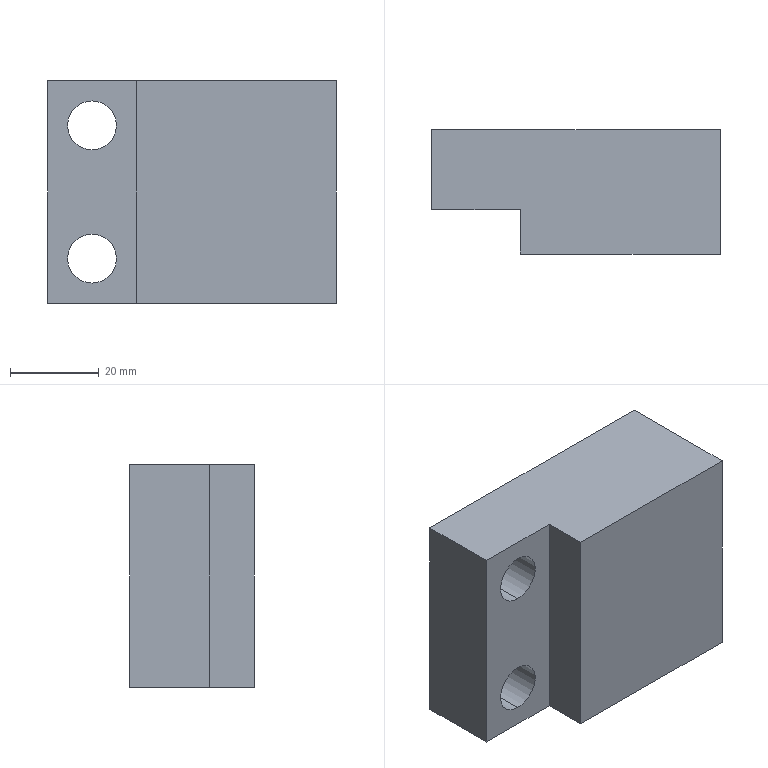Part | STEP file | OP10-025_stopper base | 1 solid | 20 faces | box 65 x 28 x 50 mm | volume 72632 mm3 | cylinder 8 | plane 8 | cone 4 | commonest cylinder face diameters 10.2 x4 11 x4
STEP:
#1=CARTESIAN_POINT('',(0.,0.,0.));
#2=DIRECTION('',(0.,0.,1.));
#3=DIRECTION('',(1.,0.,0.));
#4=AXIS2_PLACEMENT_3D('',#1,#2,#3);
#5=CARTESIAN_POINT('',(3.25,14.,7.9));
#6=VERTEX_POINT('',#5);
#7=CARTESIAN_POINT('',(32.5,14.,7.9));
#8=VERTEX_POINT('',#7);
#9=CARTESIAN_POINT('',(32.5,14.,7.9));
#10=DIRECTION('',(1.,0.,0.));
#11=VECTOR('',#10,1.);
#12=LINE('',#9,#11);
#13=CARTESIAN_POINT('',(32.5,14.,13.));
#14=DIRECTION('',(1.,0.,0.));
#15=DIRECTION('',(0.,0.,-1.));
#16=AXIS2_PLACEMENT_3D('',#13,#14,#15);
#17=CYLINDRICAL_SURFACE('',#16,5.1);
#18=CARTESIAN_POINT('',(6.283,0.));
#19=DIRECTION('',(0.,1.));
#20=VECTOR('',#19,1.);
#21=LINE('',#18,#20);
#22=(GEOMETRIC_REPRESENTATION_CONTEXT(2)PARAMETRIC_REPRESENTATION_CONTEXT()REPRESENTATION_CONTEXT('',''));
#23=DEFINITIONAL_REPRESENTATION('',(#21),#22);
#24=PCURVE('',#17,#23);
#25=CARTESIAN_POINT('',(32.5,14.,13.));
#26=DIRECTION('',(1.,0.,0.));
#27=DIRECTION('',(0.,0.,-1.));
#28=AXIS2_PLACEMENT_3D('',#25,#26,#27);
#29=CYLINDRICAL_SURFACE('',#28,5.1);
#30=CARTESIAN_POINT('',(0.,0.));
#31=DIRECTION('',(0.,1.));
#32=VECTOR('',#31,1.);
#33=LINE('',#30,#32);
#34=(GEOMETRIC_REPRESENTATION_CONTEXT(2)PARAMETRIC_REPRESENTATION_CONTEXT()REPRESENTATION_CONTEXT('',''));
#35=DEFINITIONAL_REPRESENTATION('',(#33),#34);
#36=PCURVE('',#29,#35);
#37=SURFACE_CURVE('',#12,(#24,#36),.PCURVE_S1.);
#38=EDGE_CURVE('',#6,#8,#37,.T.);
#39=ORIENTED_EDGE('',*,*,#38,.T.);
#40=CARTESIAN_POINT('',(32.5,14.,18.1));
#41=VERTEX_POINT('',#40);
#42=CARTESIAN_POINT('',(32.5,14.,13.));
#43=DIRECTION('',(1.,0.,0.));
#44=DIRECTION('',(0.,0.,-1.));
#45=AXIS2_PLACEMENT_3D('',#42,#43,#44);
#46=CIRCLE('',#45,5.1);
#47=CARTESIAN_POINT('',(0.,0.));
#48=DIRECTION('',(1.,0.));
#49=VECTOR('',#48,1.);
#50=LINE('',#47,#49);
#51=(GEOMETRIC_REPRESENTATION_CONTEXT(2)PARAMETRIC_REPRESENTATION_CONTEXT()REPRESENTATION_CONTEXT('',''));
#52=DEFINITIONAL_REPRESENTATION('',(#50),#51);
#53=PCURVE('',#17,#52);
#54=CARTESIAN_POINT('',(32.5,28.,25.));
#55=DIRECTION('',(-1.,0.,0.));
#56=DIRECTION('',(0.,0.,1.));
#57=AXIS2_PLACEMENT_3D('',#54,#55,#56);
#58=PLANE('',#57);
#59=CARTESIAN_POINT('',(-17.1,-14.));
#60=CARTESIAN_POINT('',(-17.1,-5.167));
#61=CARTESIAN_POINT('',(-9.45,-9.583));
#62=CARTESIAN_POINT('',(-1.8,-14.));
#63=CARTESIAN_POINT('',(-9.45,-18.417));
#64=CARTESIAN_POINT('',(-17.1,-22.833));
#65=CARTESIAN_POINT('',(-17.1,-14.));
#66=(BOUNDED_CURVE()B_SPLINE_CURVE(2,(#59,#60,#61,#62,#63,#64,#65),.UNSPECIFIED.,.T.,.F.)B_SPLINE_CURVE_WITH_KNOTS((1,2,2,2,2,1),(-2.094,0.,2.094,4.189,6.283,8.378),.UNSPECIFIED.)CURVE()GEOMETRIC_REPRESENTATION_ITEM()RATIONAL_B_SPLINE_CURVE((1.,0.5,1.,0.5,1.,0.5,1.))REPRESENTATION_ITEM(''));
#67=(GEOMETRIC_REPRESENTATION_CONTEXT(2)PARAMETRIC_REPRESENTATION_CONTEXT()REPRESENTATION_CONTEXT('',''));
#68=DEFINITIONAL_REPRESENTATION('',(#66),#67);
#69=PCURVE('',#58,#68);
#70=SURFACE_CURVE('',#46,(#53,#69),.PCURVE_S1.);
#71=EDGE_CURVE('',#41,#8,#70,.T.);
#72=ORIENTED_EDGE('',*,*,#71,.F.);
#73=CARTESIAN_POINT('',(3.25,14.,18.1));
#74=VERTEX_POINT('',#73);
#75=CARTESIAN_POINT('',(32.5,14.,18.1));
#76=DIRECTION('',(1.,0.,0.));
#77=VECTOR('',#76,1.);
#78=LINE('',#75,#77);
#79=CARTESIAN_POINT('',(3.142,0.));
#80=DIRECTION('',(0.,1.));
#81=VECTOR('',#80,1.);
#82=LINE('',#79,#81);
#83=(GEOMETRIC_REPRESENTATION_CONTEXT(2)PARAMETRIC_REPRESENTATION_CONTEXT()REPRESENTATION_CONTEXT('',''));
#84=DEFINITIONAL_REPRESENTATION('',(#82),#83);
#85=PCURVE('',#17,#84);
#86=CARTESIAN_POINT('',(3.142,0.));
#87=DIRECTION('',(0.,1.));
#88=VECTOR('',#87,1.);
#89=LINE('',#86,#88);
#90=(GEOMETRIC_REPRESENTATION_CONTEXT(2)PARAMETRIC_REPRESENTATION_CONTEXT()REPRESENTATION_CONTEXT('',''));
#91=DEFINITIONAL_REPRESENTATION('',(#89),#90);
#92=PCURVE('',#29,#91);
#93=SURFACE_CURVE('',#78,(#85,#92),.PCURVE_S1.);
#94=EDGE_CURVE('',#74,#41,#93,.T.);
#95=ORIENTED_EDGE('',*,*,#94,.F.);
#96=CARTESIAN_POINT('',(3.25,14.,13.));
#97=DIRECTION('',(1.,0.,0.));
#98=DIRECTION('',(0.,0.,-1.));
#99=AXIS2_PLACEMENT_3D('',#96,#97,#98);
#100=CIRCLE('',#99,5.1);
#101=CARTESIAN_POINT('',(0.,-29.25));
#102=DIRECTION('',(1.,0.));
#103=VECTOR('',#102,1.);
#104=LINE('',#101,#103);
#105=(GEOMETRIC_REPRESENTATION_CONTEXT(2)PARAMETRIC_REPRESENTATION_CONTEXT()REPRESENTATION_CONTEXT('',''));
#106=DEFINITIONAL_REPRESENTATION('',(#104),#105);
#107=PCURVE('',#17,#106);
#108=CARTESIAN_POINT('',(3.25,14.,13.));
#109=DIRECTION('',(1.,0.,0.));
#110=DIRECTION('',(0.,0.,-1.));
#111=AXIS2_PLACEMENT_3D('',#108,#109,#110);
#112=CONICAL_SURFACE('',#111,5.1,1.03);
#113=CARTESIAN_POINT('',(0.,0.));
#114=DIRECTION('',(1.,0.));
#115=VECTOR('',#114,1.);
#116=LINE('',#113,#115);
#117=(GEOMETRIC_REPRESENTATION_CONTEXT(2)PARAMETRIC_REPRESENTATION_CONTEXT()REPRESENTATION_CONTEXT('',''));
#118=DEFINITIONAL_REPRESENTATION('',(#116),#117);
#119=PCURVE('',#112,#118);
#120=SURFACE_CURVE('',#100,(#107,#119),.PCURVE_S1.);
#121=EDGE_CURVE('',#74,#6,#120,.T.);
#122=ORIENTED_EDGE('',*,*,#121,.T.);
#123=EDGE_LOOP('',(#39,#72,#95,#122));
#124=FACE_BOUND('',#123,.F.);
#125=ADVANCED_FACE('',(#124),#17,.F.);
#126=ORIENTED_EDGE('',*,*,#121,.F.);
#127=CARTESIAN_POINT('',(0.1856,14.,13.));
#128=VERTEX_POINT('',#127);
#129=CARTESIAN_POINT('',(3.25,14.,18.1));
#130=DIRECTION('',(0.515,0.,0.8572));
#131=VECTOR('',#130,1.);
#132=LINE('',#129,#131);
#133=CARTESIAN_POINT('',(3.142,0.));
#134=DIRECTION('',(0.,1.));
#135=VECTOR('',#134,1.);
#136=LINE('',#133,#135);
#137=(GEOMETRIC_REPRESENTATION_CONTEXT(2)PARAMETRIC_REPRESENTATION_CONTEXT()REPRESENTATION_CONTEXT('',''));
#138=DEFINITIONAL_REPRESENTATION('',(#136),#137);
#139=PCURVE('',#112,#138);
#140=CARTESIAN_POINT('',(3.25,14.,13.));
#141=DIRECTION('',(1.,0.,0.));
#142=DIRECTION('',(0.,0.,-1.));
#143=AXIS2_PLACEMENT_3D('',#140,#141,#142);
#144=CONICAL_SURFACE('',#143,5.1,1.03);
#145=CARTESIAN_POINT('',(3.142,0.));
#146=DIRECTION('',(0.,1.));
#147=VECTOR('',#146,1.);
#148=LINE('',#145,#147);
#149=(GEOMETRIC_REPRESENTATION_CONTEXT(2)PARAMETRIC_REPRESENTATION_CONTEXT()REPRESENTATION_CONTEXT('',''));
#150=DEFINITIONAL_REPRESENTATION('',(#148),#149);
#151=PCURVE('',#144,#150);
#152=SURFACE_CURVE('',#132,(#139,#151),.PCURVE_S1.);
#153=EDGE_CURVE('',#128,#74,#152,.T.);
#154=ORIENTED_EDGE('',*,*,#153,.F.);
#155=CARTESIAN_POINT('',(3.25,14.,7.9));
#156=DIRECTION('',(0.515,0.,-0.8572));
#157=VECTOR('',#156,1.);
#158=LINE('',#155,#157);
#159=CARTESIAN_POINT('',(6.283,0.));
#160=DIRECTION('',(0.,1.));
#161=VECTOR('',#160,1.);
#162=LINE('',#159,#161);
#163=(GEOMETRIC_REPRESENTATION_CONTEXT(2)PARAMETRIC_REPRESENTATION_CONTEXT()REPRESENTATION_CONTEXT('',''));
#164=DEFINITIONAL_REPRESENTATION('',(#162),#163);
#165=PCURVE('',#112,#164);
#166=CARTESIAN_POINT('',(0.,0.));
#167=DIRECTION('',(0.,1.));
#168=VECTOR('',#167,1.);
#169=LINE('',#166,#168);
#170=(GEOMETRIC_REPRESENTATION_CONTEXT(2)PARAMETRIC_REPRESENTATION_CONTEXT()REPRESENTATION_CONTEXT('',''));
#171=DEFINITIONAL_REPRESENTATION('',(#169),#170);
#172=PCURVE('',#144,#171);
#173=SURFACE_CURVE('',#158,(#165,#172),.PCURVE_S1.);
#174=EDGE_CURVE('',#128,#6,#173,.T.);
#175=ORIENTED_EDGE('',*,*,#174,.T.);
#176=EDGE_LOOP('',(#126,#154,#175));
#177=FACE_BOUND('',#176,.F.);
#178=ADVANCED_FACE('',(#177),#112,.F.);
#179=CARTESIAN_POINT('',(3.25,14.,-18.1));
#180=VERTEX_POINT('',#179);
#181=CARTESIAN_POINT('',(32.5,14.,-18.1));
#182=VERTEX_POINT('',#181);
#183=CARTESIAN_POINT('',(32.5,14.,-18.1));
#184=DIRECTION('',(1.,0.,0.));
#185=VECTOR('',#184,1.);
#186=LINE('',#183,#185);
#187=CARTESIAN_POINT('',(32.5,14.,-13.));
#188=DIRECTION('',(1.,0.,0.));
#189=DIRECTION('',(0.,0.,-1.));
#190=AXIS2_PLACEMENT_3D('',#187,#188,#189);
#191=CYLINDRICAL_SURFACE('',#190,5.1);
#192=CARTESIAN_POINT('',(6.283,0.));
#193=DIRECTION('',(0.,1.));
#194=VECTOR('',#193,1.);
#195=LINE('',#192,#194);
#196=(GEOMETRIC_REPRESENTATION_CONTEXT(2)PARAMETRIC_REPRESENTATION_CONTEXT()REPRESENTATION_CONTEXT('',''));
#197=DEFINITIONAL_REPRESENTATION('',(#195),#196);
#198=PCURVE('',#191,#197);
#199=CARTESIAN_POINT('',(32.5,14.,-13.));
#200=DIRECTION('',(1.,0.,0.));
#201=DIRECTION('',(0.,0.,-1.));
#202=AXIS2_PLACEMENT_3D('',#199,#200,#201);
#203=CYLINDRICAL_SURFACE('',#202,5.1);
#204=CARTESIAN_POINT('',(0.,0.));
#205=DIRECTION('',(0.,1.));
#206=VECTOR('',#205,1.);
#207=LINE('',#204,#206);
#208=(GEOMETRIC_REPRESENTATION_CONTEXT(2)PARAMETRIC_REPRESENTATION_CONTEXT()REPRESENTATION_CONTEXT('',''));
#209=DEFINITIONAL_REPRESENTATION('',(#207),#208);
#210=PCURVE('',#203,#209);
#211=SURFACE_CURVE('',#186,(#198,#210),.PCURVE_S1.);
#212=EDGE_CURVE('',#180,#182,#211,.T.);
#213=ORIENTED_EDGE('',*,*,#212,.T.);
#214=CARTESIAN_POINT('',(32.5,14.,-7.9));
#215=VERTEX_POINT('',#214);
#216=CARTESIAN_POINT('',(32.5,14.,-13.));
#217=DIRECTION('',(1.,0.,0.));
#218=DIRECTION('',(0.,0.,-1.));
#219=AXIS2_PLACEMENT_3D('',#216,#217,#218);
#220=CIRCLE('',#219,5.1);
#221=CARTESIAN_POINT('',(0.,0.));
#222=DIRECTION('',(1.,0.));
#223=VECTOR('',#222,1.);
#224=LINE('',#221,#223);
#225=(GEOMETRIC_REPRESENTATION_CONTEXT(2)PARAMETRIC_REPRESENTATION_CONTEXT()REPRESENTATION_CONTEXT('',''));
#226=DEFINITIONAL_REPRESENTATION('',(#224),#225);
#227=PCURVE('',#191,#226);
#228=CARTESIAN_POINT('',(-43.1,-14.));
#229=CARTESIAN_POINT('',(-43.1,-5.167));
#230=CARTESIAN_POINT('',(-35.45,-9.583));
#231=CARTESIAN_POINT('',(-27.8,-14.));
#232=CARTESIAN_POINT('',(-35.45,-18.417));
#233=CARTESIAN_POINT('',(-43.1,-22.833));
#234=CARTESIAN_POINT('',(-43.1,-14.));
#235=(BOUNDED_CURVE()B_SPLINE_CURVE(2,(#228,#229,#230,#231,#232,#233,#234),.UNSPECIFIED.,.T.,.F.)B_SPLINE_CURVE_WITH_KNOTS((1,2,2,2,2,1),(-2.094,0.,2.094,4.189,6.283,8.378),.UNSPECIFIED.)CURVE()GEOMETRIC_REPRESENTATION_ITEM()RATIONAL_B_SPLINE_CURVE((1.,0.5,1.,0.5,1.,0.5,1.))REPRESENTATION_ITEM(''));
#236=(GEOMETRIC_REPRESENTATION_CONTEXT(2)PARAMETRIC_REPRESENTATION_CONTEXT()REPRESENTATION_CONTEXT('',''));
#237=DEFINITIONAL_REPRESENTATION('',(#235),#236);
#238=PCURVE('',#58,#237);
#239=SURFACE_CURVE('',#220,(#227,#238),.PCURVE_S1.);
#240=EDGE_CURVE('',#215,#182,#239,.T.);
#241=ORIENTED_EDGE('',*,*,#240,.F.);
#242=CARTESIAN_POINT('',(3.25,14.,-7.9));
#243=VERTEX_POINT('',#242);
#244=CARTESIAN_POINT('',(32.5,14.,-7.9));
#245=DIRECTION('',(1.,0.,0.));
#246=VECTOR('',#245,1.);
#247=LINE('',#244,#246);
#248=CARTESIAN_POINT('',(3.142,0.));
#249=DIRECTION('',(0.,1.));
#250=VECTOR('',#249,1.);
#251=LINE('',#248,#250);
#252=(GEOMETRIC_REPRESENTATION_CONTEXT(2)PARAMETRIC_REPRESENTATION_CONTEXT()REPRESENTATION_CONTEXT('',''));
#253=DEFINITIONAL_REPRESENTATION('',(#251),#252);
#254=PCURVE('',#191,#253);
#255=CARTESIAN_POINT('',(3.142,0.));
#256=DIRECTION('',(0.,1.));
#257=VECTOR('',#256,1.);
#258=LINE('',#255,#257);
#259=(GEOMETRIC_REPRESENTATION_CONTEXT(2)PARAMETRIC_REPRESENTATION_CONTEXT()REPRESENTATION_CONTEXT('',''));
#260=DEFINITIONAL_REPRESENTATION('',(#258),#259);
#261=PCURVE('',#203,#260);
#262=SURFACE_CURVE('',#247,(#254,#261),.PCURVE_S1.);
#263=EDGE_CURVE('',#243,#215,#262,.T.);
#264=ORIENTED_EDGE('',*,*,#263,.F.);
#265=CARTESIAN_POINT('',(3.25,14.,-13.));
#266=DIRECTION('',(1.,0.,0.));
#267=DIRECTION('',(0.,0.,-1.));
#268=AXIS2_PLACEMENT_3D('',#265,#266,#267);
#269=CIRCLE('',#268,5.1);
#270=CARTESIAN_POINT('',(0.,-29.25));
#271=DIRECTION('',(1.,0.));
#272=VECTOR('',#271,1.);
#273=LINE('',#270,#272);
#274=(GEOMETRIC_REPRESENTATION_CONTEXT(2)PARAMETRIC_REPRESENTATION_CONTEXT()REPRESENTATION_CONTEXT('',''));
#275=DEFINITIONAL_REPRESENTATION('',(#273),#274);
#276=PCURVE('',#191,#275);
#277=CARTESIAN_POINT('',(3.25,14.,-13.));
#278=DIRECTION('',(1.,0.,0.));
#279=DIRECTION('',(0.,0.,-1.));
#280=AXIS2_PLACEMENT_3D('',#277,#278,#279);
#281=CONICAL_SURFACE('',#280,5.1,1.03);
#282=CARTESIAN_POINT('',(0.,0.));
#283=DIRECTION('',(1.,0.));
#284=VECTOR('',#283,1.);
#285=LINE('',#282,#284);
#286=(GEOMETRIC_REPRESENTATION_CONTEXT(2)PARAMETRIC_REPRESENTATION_CONTEXT()REPRESENTATION_CONTEXT('',''));
#287=DEFINITIONAL_REPRESENTATION('',(#285),#286);
#288=PCURVE('',#281,#287);
#289=SURFACE_CURVE('',#269,(#276,#288),.PCURVE_S1.);
#290=EDGE_CURVE('',#243,#180,#289,.T.);
#291=ORIENTED_EDGE('',*,*,#290,.T.);
#292=EDGE_LOOP('',(#213,#241,#264,#291));
#293=FACE_BOUND('',#292,.F.);
#294=ADVANCED_FACE('',(#293),#191,.F.);
#295=ORIENTED_EDGE('',*,*,#290,.F.);
#296=CARTESIAN_POINT('',(0.1856,14.,-13.));
#297=VERTEX_POINT('',#296);
#298=CARTESIAN_POINT('',(3.25,14.,-7.9));
#299=DIRECTION('',(0.515,0.,0.8572));
#300=VECTOR('',#299,1.);
#301=LINE('',#298,#300);
#302=CARTESIAN_POINT('',(3.142,0.));
#303=DIRECTION('',(0.,1.));
#304=VECTOR('',#303,1.);
#305=LINE('',#302,#304);
#306=(GEOMETRIC_REPRESENTATION_CONTEXT(2)PARAMETRIC_REPRESENTATION_CONTEXT()REPRESENTATION_CONTEXT('',''));
#307=DEFINITIONAL_REPRESENTATION('',(#305),#306);
#308=PCURVE('',#281,#307);
#309=CARTESIAN_POINT('',(3.25,14.,-13.));
#310=DIRECTION('',(1.,0.,0.));
#311=DIRECTION('',(0.,0.,-1.));
#312=AXIS2_PLACEMENT_3D('',#309,#310,#311);
#313=CONICAL_SURFACE('',#312,5.1,1.03);
#314=CARTESIAN_POINT('',(3.142,0.));
#315=DIRECTION('',(0.,1.));
#316=VECTOR('',#315,1.);
#317=LINE('',#314,#316);
#318=(GEOMETRIC_REPRESENTATION_CONTEXT(2)PARAMETRIC_REPRESENTATION_CONTEXT()REPRESENTATION_CONTEXT('',''));
#319=DEFINITIONAL_REPRESENTATION('',(#317),#318);
#320=PCURVE('',#313,#319);
#321=SURFACE_CURVE('',#301,(#308,#320),.PCURVE_S1.);
#322=EDGE_CURVE('',#297,#243,#321,.T.);
#323=ORIENTED_EDGE('',*,*,#322,.F.);
#324=CARTESIAN_POINT('',(3.25,14.,-18.1));
#325=DIRECTION('',(0.515,0.,-0.8572));
#326=VECTOR('',#325,1.);
#327=LINE('',#324,#326);
#328=CARTESIAN_POINT('',(6.283,0.));
#329=DIRECTION('',(0.,1.));
#330=VECTOR('',#329,1.);
#331=LINE('',#328,#330);
#332=(GEOMETRIC_REPRESENTATION_CONTEXT(2)PARAMETRIC_REPRESENTATION_CONTEXT()REPRESENTATION_CONTEXT('',''));
#333=DEFINITIONAL_REPRESENTATION('',(#331),#332);
#334=PCURVE('',#281,#333);
#335=CARTESIAN_POINT('',(0.,0.));
#336=DIRECTION('',(0.,1.));
#337=VECTOR('',#336,1.);
#338=LINE('',#335,#337);
#339=(GEOMETRIC_REPRESENTATION_CONTEXT(2)PARAMETRIC_REPRESENTATION_CONTEXT()REPRESENTATION_CONTEXT('',''));
#340=DEFINITIONAL_REPRESENTATION('',(#338),#339);
#341=PCURVE('',#313,#340);
#342=SURFACE_CURVE('',#327,(#334,#341),.PCURVE_S1.);
#343=EDGE_CURVE('',#297,#180,#342,.T.);
#344=ORIENTED_EDGE('',*,*,#343,.T.);
#345=EDGE_LOOP('',(#295,#323,#344));
#346=FACE_BOUND('',#345,.F.);
#347=ADVANCED_FACE('',(#346),#281,.F.);
#348=CARTESIAN_POINT('',(-22.5,28.,9.5));
#349=VERTEX_POINT('',#348);
#350=CARTESIAN_POINT('',(-22.5,10.,9.5));
#351=VERTEX_POINT('',#350);
#352=CARTESIAN_POINT('',(-22.5,28.,9.5));
#353=DIRECTION('',(0.,-1.,0.));
#354=VECTOR('',#353,1.);
#355=LINE('',#352,#354);
#356=CARTESIAN_POINT('',(-22.5,28.,15.));
#357=DIRECTION('',(0.,-1.,0.));
#358=DIRECTION('',(0.,0.,-1.));
#359=AXIS2_PLACEMENT_3D('',#356,#357,#358);
#360=CYLINDRICAL_SURFACE('',#359,5.5);
#361=CARTESIAN_POINT('',(6.283,0.));
#362=DIRECTION('',(0.,1.));
#363=VECTOR('',#362,1.);
#364=LINE('',#361,#363);
#365=(GEOMETRIC_REPRESENTATION_CONTEXT(2)PARAMETRIC_REPRESENTATION_CONTEXT()REPRESENTATION_CONTEXT('',''));
#366=DEFINITIONAL_REPRESENTATION('',(#364),#365);
#367=PCURVE('',#360,#366);
#368=CARTESIAN_POINT('',(-22.5,28.,15.));
#369=DIRECTION('',(0.,-1.,0.));
#370=DIRECTION('',(0.,0.,-1.));
#371=AXIS2_PLACEMENT_3D('',#368,#369,#370);
#372=CYLINDRICAL_SURFACE('',#371,5.5);
#373=CARTESIAN_POINT('',(0.,0.));
#374=DIRECTION('',(0.,1.));
#375=VECTOR('',#374,1.);
#376=LINE('',#373,#375);
#377=(GEOMETRIC_REPRESENTATION_CONTEXT(2)PARAMETRIC_REPRESENTATION_CONTEXT()REPRESENTATION_CONTEXT('',''));
#378=DEFINITIONAL_REPRESENTATION('',(#376),#377);
#379=PCURVE('',#372,#378);
#380=SURFACE_CURVE('',#355,(#367,#379),.PCURVE_S1.);
#381=EDGE_CURVE('',#349,#351,#380,.T.);
#382=ORIENTED_EDGE('',*,*,#381,.T.);
#383=CARTESIAN_POINT('',(-22.5,10.,20.5));
#384=VERTEX_POINT('',#383);
#385=CARTESIAN_POINT('',(-22.5,10.,15.));
#386=DIRECTION('',(0.,1.,0.));
#387=DIRECTION('',(0.,0.,1.));
#388=AXIS2_PLACEMENT_3D('',#385,#386,#387);
#389=CIRCLE('',#388,5.5);
#390=CARTESIAN_POINT('',(9.425,18.));
#391=DIRECTION('',(-1.,0.));
#392=VECTOR('',#391,1.);
#393=LINE('',#390,#392);
#394=(GEOMETRIC_REPRESENTATION_CONTEXT(2)PARAMETRIC_REPRESENTATION_CONTEXT()REPRESENTATION_CONTEXT('',''));
#395=DEFINITIONAL_REPRESENTATION('',(#393),#394);
#396=PCURVE('',#360,#395);
#397=CARTESIAN_POINT('',(-32.5,10.,-33.));
#398=DIRECTION('',(0.,1.,0.));
#399=DIRECTION('',(0.,0.,1.));
#400=AXIS2_PLACEMENT_3D('',#397,#398,#399);
#401=PLANE('',#400);
#402=CARTESIAN_POINT('',(48.,10.));
#403=DIRECTION('',(1.,0.));
#404=AXIS2_PLACEMENT_2D('',#402,#403);
#405=CIRCLE('',#404,5.5);
#406=(GEOMETRIC_REPRESENTATION_CONTEXT(2)PARAMETRIC_REPRESENTATION_CONTEXT()REPRESENTATION_CONTEXT('',''));
#407=DEFINITIONAL_REPRESENTATION('',(#405),#406);
#408=PCURVE('',#401,#407);
#409=SURFACE_CURVE('',#389,(#396,#408),.PCURVE_S1.);
#410=EDGE_CURVE('',#351,#384,#409,.T.);
#411=ORIENTED_EDGE('',*,*,#410,.T.);
#412=CARTESIAN_POINT('',(-22.5,28.,20.5));
#413=VERTEX_POINT('',#412);
#414=CARTESIAN_POINT('',(-22.5,28.,20.5));
#415=DIRECTION('',(0.,-1.,0.));
#416=VECTOR('',#415,1.);
#417=LINE('',#414,#416);
#418=CARTESIAN_POINT('',(3.142,0.));
#419=DIRECTION('',(0.,1.));
#420=VECTOR('',#419,1.);
#421=LINE('',#418,#420);
#422=(GEOMETRIC_REPRESENTATION_CONTEXT(2)PARAMETRIC_REPRESENTATION_CONTEXT()REPRESENTATION_CONTEXT('',''));
#423=DEFINITIONAL_REPRESENTATION('',(#421),#422);
#424=PCURVE('',#360,#423);
#425=CARTESIAN_POINT('',(3.142,0.));
#426=DIRECTION('',(0.,1.));
#427=VECTOR('',#426,1.);
#428=LINE('',#425,#427);
#429=(GEOMETRIC_REPRESENTATION_CONTEXT(2)PARAMETRIC_REPRESENTATION_CONTEXT()REPRESENTATION_CONTEXT('',''));
#430=DEFINITIONAL_REPRESENTATION('',(#428),#429);
#431=PCURVE('',#372,#430);
#432=SURFACE_CURVE('',#417,(#424,#431),.PCURVE_S1.);
#433=EDGE_CURVE('',#413,#384,#432,.T.);
#434=ORIENTED_EDGE('',*,*,#433,.F.);
#435=CARTESIAN_POINT('',(-22.5,28.,15.));
#436=DIRECTION('',(0.,1.,0.));
#437=DIRECTION('',(0.,0.,1.));
#438=AXIS2_PLACEMENT_3D('',#435,#436,#437);
#439=CIRCLE('',#438,5.5);
#440=CARTESIAN_POINT('',(9.425,0.));
#441=DIRECTION('',(-1.,0.));
#442=VECTOR('',#441,1.);
#443=LINE('',#440,#442);
#444=(GEOMETRIC_REPRESENTATION_CONTEXT(2)PARAMETRIC_REPRESENTATION_CONTEXT()REPRESENTATION_CONTEXT('',''));
#445=DEFINITIONAL_REPRESENTATION('',(#443),#444);
#446=PCURVE('',#360,#445);
#447=CARTESIAN_POINT('',(0.,28.,0.));
#448=DIRECTION('',(0.,-1.,0.));
#449=DIRECTION('',(0.,0.,-1.));
#450=AXIS2_PLACEMENT_3D('',#447,#448,#449);
#451=PLANE('',#450);
#452=CARTESIAN_POINT('',(-20.5,-22.5));
#453=CARTESIAN_POINT('',(-20.5,-12.974));
#454=CARTESIAN_POINT('',(-12.25,-17.737));
#455=CARTESIAN_POINT('',(-4.,-22.5));
#456=CARTESIAN_POINT('',(-12.25,-27.263));
#457=CARTESIAN_POINT('',(-20.5,-32.026));
#458=CARTESIAN_POINT('',(-20.5,-22.5));
#459=(BOUNDED_CURVE()B_SPLINE_CURVE(2,(#452,#453,#454,#455,#456,#457,#458),.UNSPECIFIED.,.T.,.F.)B_SPLINE_CURVE_WITH_KNOTS((1,2,2,2,2,1),(-2.094,0.,2.094,4.189,6.283,8.378),.UNSPECIFIED.)CURVE()GEOMETRIC_REPRESENTATION_ITEM()RATIONAL_B_SPLINE_CURVE((1.,0.5,1.,0.5,1.,0.5,1.))REPRESENTATION_ITEM(''));
#460=(GEOMETRIC_REPRESENTATION_CONTEXT(2)PARAMETRIC_REPRESENTATION_CONTEXT()REPRESENTATION_CONTEXT('',''));
#461=DEFINITIONAL_REPRESENTATION('',(#459),#460);
#462=PCURVE('',#451,#461);
#463=SURFACE_CURVE('',#439,(#446,#462),.PCURVE_S1.);
#464=EDGE_CURVE('',#349,#413,#463,.T.);
#465=ORIENTED_EDGE('',*,*,#464,.F.);
#466=EDGE_LOOP('',(#382,#411,#434,#465));
#467=FACE_BOUND('',#466,.F.);
#468=ADVANCED_FACE('',(#467),#360,.F.);
#469=CARTESIAN_POINT('',(-22.5,28.,-20.5));
#470=VERTEX_POINT('',#469);
#471=CARTESIAN_POINT('',(-22.5,10.,-20.5));
#472=VERTEX_POINT('',#471);
#473=CARTESIAN_POINT('',(-22.5,28.,-20.5));
#474=DIRECTION('',(0.,-1.,0.));
#475=VECTOR('',#474,1.);
#476=LINE('',#473,#475);
#477=CARTESIAN_POINT('',(-22.5,28.,-15.));
#478=DIRECTION('',(0.,-1.,0.));
#479=DIRECTION('',(0.,0.,-1.));
#480=AXIS2_PLACEMENT_3D('',#477,#478,#479);
#481=CYLINDRICAL_SURFACE('',#480,5.5);
#482=CARTESIAN_POINT('',(6.283,0.));
#483=DIRECTION('',(0.,1.));
#484=VECTOR('',#483,1.);
#485=LINE('',#482,#484);
#486=(GEOMETRIC_REPRESENTATION_CONTEXT(2)PARAMETRIC_REPRESENTATION_CONTEXT()REPRESENTATION_CONTEXT('',''));
#487=DEFINITIONAL_REPRESENTATION('',(#485),#486);
#488=PCURVE('',#481,#487);
#489=CARTESIAN_POINT('',(-22.5,28.,-15.));
#490=DIRECTION('',(0.,-1.,0.));
#491=DIRECTION('',(0.,0.,-1.));
#492=AXIS2_PLACEMENT_3D('',#489,#490,#491);
#493=CYLINDRICAL_SURFACE('',#492,5.5);
#494=CARTESIAN_POINT('',(0.,0.));
#495=DIRECTION('',(0.,1.));
#496=VECTOR('',#495,1.);
#497=LINE('',#494,#496);
#498=(GEOMETRIC_REPRESENTATION_CONTEXT(2)PARAMETRIC_REPRESENTATION_CONTEXT()REPRESENTATION_CONTEXT('',''));
#499=DEFINITIONAL_REPRESENTATION('',(#497),#498);
#500=PCURVE('',#493,#499);
#501=SURFACE_CURVE('',#476,(#488,#500),.PCURVE_S1.);
#502=EDGE_CURVE('',#470,#472,#501,.T.);
#503=ORIENTED_EDGE('',*,*,#502,.T.);
#504=CARTESIAN_POINT('',(-22.5,10.,-9.5));
#505=VERTEX_POINT('',#504);
#506=CARTESIAN_POINT('',(-22.5,10.,-15.));
#507=DIRECTION('',(0.,1.,0.));
#508=DIRECTION('',(0.,0.,1.));
#509=AXIS2_PLACEMENT_3D('',#506,#507,#508);
#510=CIRCLE('',#509,5.5);
#511=CARTESIAN_POINT('',(9.425,18.));
#512=DIRECTION('',(-1.,0.));
#513=VECTOR('',#512,1.);
#514=LINE('',#511,#513);
#515=(GEOMETRIC_REPRESENTATION_CONTEXT(2)PARAMETRIC_REPRESENTATION_CONTEXT()REPRESENTATION_CONTEXT('',''));
#516=DEFINITIONAL_REPRESENTATION('',(#514),#515);
#517=PCURVE('',#481,#516);
#518=CARTESIAN_POINT('',(18.,10.));
#519=DIRECTION('',(1.,0.));
#520=AXIS2_PLACEMENT_2D('',#518,#519);
#521=CIRCLE('',#520,5.5);
#522=(GEOMETRIC_REPRESENTATION_CONTEXT(2)PARAMETRIC_REPRESENTATION_CONTEXT()REPRESENTATION_CONTEXT('',''));
#523=DEFINITIONAL_REPRESENTATION('',(#521),#522);
#524=PCURVE('',#401,#523);
#525=SURFACE_CURVE('',#510,(#517,#524),.PCURVE_S1.);
#526=EDGE_CURVE('',#472,#505,#525,.T.);
#527=ORIENTED_EDGE('',*,*,#526,.T.);
#528=CARTESIAN_POINT('',(-22.5,28.,-9.5));
#529=VERTEX_POINT('',#528);
#530=CARTESIAN_POINT('',(-22.5,28.,-9.5));
#531=DIRECTION('',(0.,-1.,0.));
#532=VECTOR('',#531,1.);
#533=LINE('',#530,#532);
#534=CARTESIAN_POINT('',(3.142,0.));
#535=DIRECTION('',(0.,1.));
#536=VECTOR('',#535,1.);
#537=LINE('',#534,#536);
#538=(GEOMETRIC_REPRESENTATION_CONTEXT(2)PARAMETRIC_REPRESENTATION_CONTEXT()REPRESENTATION_CONTEXT('',''));
#539=DEFINITIONAL_REPRESENTATION('',(#537),#538);
#540=PCURVE('',#481,#539);
#541=CARTESIAN_POINT('',(3.142,0.));
#542=DIRECTION('',(0.,1.));
#543=VECTOR('',#542,1.);
#544=LINE('',#541,#543);
#545=(GEOMETRIC_REPRESENTATION_CONTEXT(2)PARAMETRIC_REPRESENTATION_CONTEXT()REPRESENTATION_CONTEXT('',''));
#546=DEFINITIONAL_REPRESENTATION('',(#544),#545);
#547=PCURVE('',#493,#546);
#548=SURFACE_CURVE('',#533,(#540,#547),.PCURVE_S1.);
#549=EDGE_CURVE('',#529,#505,#548,.T.);
#550=ORIENTED_EDGE('',*,*,#549,.F.);
#551=CARTESIAN_POINT('',(-22.5,28.,-15.));
#552=DIRECTION('',(0.,1.,0.));
#553=DIRECTION('',(0.,0.,1.));
#554=AXIS2_PLACEMENT_3D('',#551,#552,#553);
#555=CIRCLE('',#554,5.5);
#556=CARTESIAN_POINT('',(9.425,0.));
#557=DIRECTION('',(-1.,0.));
#558=VECTOR('',#557,1.);
#559=LINE('',#556,#558);
#560=(GEOMETRIC_REPRESENTATION_CONTEXT(2)PARAMETRIC_REPRESENTATION_CONTEXT()REPRESENTATION_CONTEXT('',''));
#561=DEFINITIONAL_REPRESENTATION('',(#559),#560);
#562=PCURVE('',#481,#561);
#563=CARTESIAN_POINT('',(9.5,-22.5));
#564=CARTESIAN_POINT('',(9.5,-12.974));
#565=CARTESIAN_POINT('',(17.75,-17.737));
#566=CARTESIAN_POINT('',(26.,-22.5));
#567=CARTESIAN_POINT('',(17.75,-27.263));
#568=CARTESIAN_POINT('',(9.5,-32.026));
#569=CARTESIAN_POINT('',(9.5,-22.5));
#570=(BOUNDED_CURVE()B_SPLINE_CURVE(2,(#563,#564,#565,#566,#567,#568,#569),.UNSPECIFIED.,.T.,.F.)B_SPLINE_CURVE_WITH_KNOTS((1,2,2,2,2,1),(-2.094,0.,2.094,4.189,6.283,8.378),.UNSPECIFIED.)CURVE()GEOMETRIC_REPRESENTATION_ITEM()RATIONAL_B_SPLINE_CURVE((1.,0.5,1.,0.5,1.,0.5,1.))REPRESENTATION_ITEM(''));
#571=(GEOMETRIC_REPRESENTATION_CONTEXT(2)PARAMETRIC_REPRESENTATION_CONTEXT()REPRESENTATION_CONTEXT('',''));
#572=DEFINITIONAL_REPRESENTATION('',(#570),#571);
#573=PCURVE('',#451,#572);
#574=SURFACE_CURVE('',#555,(#562,#573),.PCURVE_S1.);
#575=EDGE_CURVE('',#470,#529,#574,.T.);
#576=ORIENTED_EDGE('',*,*,#575,.F.);
#577=EDGE_LOOP('',(#503,#527,#550,#576));
#578=FACE_BOUND('',#577,.F.);
#579=ADVANCED_FACE('',(#578),#481,.F.);
#580=ORIENTED_EDGE('',*,*,#575,.F.);
#581=CARTESIAN_POINT('',(-22.5,28.,-15.));
#582=DIRECTION('',(0.,1.,0.));
#583=DIRECTION('',(0.,0.,1.));
#584=AXIS2_PLACEMENT_3D('',#581,#582,#583);
#585=CIRCLE('',#584,5.5);
#586=CARTESIAN_POINT('',(9.5,-22.5));
#587=CARTESIAN_POINT('',(9.5,-12.974));
#588=CARTESIAN_POINT('',(17.75,-17.737));
#589=CARTESIAN_POINT('',(26.,-22.5));
#590=CARTESIAN_POINT('',(17.75,-27.263));
#591=CARTESIAN_POINT('',(9.5,-32.026));
#592=CARTESIAN_POINT('',(9.5,-22.5));
#593=(BOUNDED_CURVE()B_SPLINE_CURVE(2,(#586,#587,#588,#589,#590,#591,#592),.UNSPECIFIED.,.T.,.F.)B_SPLINE_CURVE_WITH_KNOTS((1,2,2,2,2,1),(-2.094,0.,2.094,4.189,6.283,8.378),.UNSPECIFIED.)CURVE()GEOMETRIC_REPRESENTATION_ITEM()RATIONAL_B_SPLINE_CURVE((1.,0.5,1.,0.5,1.,0.5,1.))REPRESENTATION_ITEM(''));
#594=(GEOMETRIC_REPRESENTATION_CONTEXT(2)PARAMETRIC_REPRESENTATION_CONTEXT()REPRESENTATION_CONTEXT('',''));
#595=DEFINITIONAL_REPRESENTATION('',(#593),#594);
#596=PCURVE('',#451,#595);
#597=CARTESIAN_POINT('',(3.142,0.));
#598=DIRECTION('',(-1.,0.));
#599=VECTOR('',#598,1.);
#600=LINE('',#597,#599);
#601=(GEOMETRIC_REPRESENTATION_CONTEXT(2)PARAMETRIC_REPRESENTATION_CONTEXT()REPRESENTATION_CONTEXT('',''));
#602=DEFINITIONAL_REPRESENTATION('',(#600),#601);
#603=PCURVE('',#493,#602);
#604=SURFACE_CURVE('',#585,(#596,#603),.PCURVE_S1.);
#605=EDGE_CURVE('',#529,#470,#604,.T.);
#606=ORIENTED_EDGE('',*,*,#605,.F.);
#607=EDGE_LOOP('',(#580,#606));
#608=FACE_BOUND('',#607,.T.);
#609=CARTESIAN_POINT('',(32.5,28.,25.));
#610=VERTEX_POINT('',#609);
#611=CARTESIAN_POINT('',(32.5,28.,-25.));
#612=VERTEX_POINT('',#611);
#613=CARTESIAN_POINT('',(32.5,28.,25.));
#614=DIRECTION('',(0.,0.,-1.));
#615=VECTOR('',#614,1.);
#616=LINE('',#613,#615);
#617=CARTESIAN_POINT('',(-25.,32.5));
#618=DIRECTION('',(1.,0.));
#619=VECTOR('',#618,1.);
#620=LINE('',#617,#619);
#621=(GEOMETRIC_REPRESENTATION_CONTEXT(2)PARAMETRIC_REPRESENTATION_CONTEXT()REPRESENTATION_CONTEXT('',''));
#622=DEFINITIONAL_REPRESENTATION('',(#620),#621);
#623=PCURVE('',#451,#622);
#624=CARTESIAN_POINT('',(0.,0.));
#625=DIRECTION('',(-1.,0.));
#626=VECTOR('',#625,1.);
#627=LINE('',#624,#626);
#628=(GEOMETRIC_REPRESENTATION_CONTEXT(2)PARAMETRIC_REPRESENTATION_CONTEXT()REPRESENTATION_CONTEXT('',''));
#629=DEFINITIONAL_REPRESENTATION('',(#627),#628);
#630=PCURVE('',#58,#629);
#631=SURFACE_CURVE('',#616,(#623,#630),.PCURVE_S1.);
#632=EDGE_CURVE('',#610,#612,#631,.T.);
#633=ORIENTED_EDGE('',*,*,#632,.T.);
#634=CARTESIAN_POINT('',(-32.5,28.,-25.));
#635=VERTEX_POINT('',#634);
#636=CARTESIAN_POINT('',(-32.5,28.,-25.));
#637=DIRECTION('',(-1.,0.,0.));
#638=VECTOR('',#637,1.);
#639=LINE('',#636,#638);
#640=CARTESIAN_POINT('',(25.,-32.5));
#641=DIRECTION('',(0.,-1.));
#642=VECTOR('',#641,1.);
#643=LINE('',#640,#642);
#644=(GEOMETRIC_REPRESENTATION_CONTEXT(2)PARAMETRIC_REPRESENTATION_CONTEXT()REPRESENTATION_CONTEXT('',''));
#645=DEFINITIONAL_REPRESENTATION('',(#643),#644);
#646=PCURVE('',#451,#645);
#647=CARTESIAN_POINT('',(-32.5,28.,-25.));
#648=DIRECTION('',(0.,0.,1.));
#649=DIRECTION('',(1.,0.,0.));
#650=AXIS2_PLACEMENT_3D('',#647,#648,#649);
#651=PLANE('',#650);
#652=CARTESIAN_POINT('',(0.,0.));
#653=DIRECTION('',(-1.,0.));
#654=VECTOR('',#653,1.);
#655=LINE('',#652,#654);
#656=(GEOMETRIC_REPRESENTATION_CONTEXT(2)PARAMETRIC_REPRESENTATION_CONTEXT()REPRESENTATION_CONTEXT('',''));
#657=DEFINITIONAL_REPRESENTATION('',(#655),#656);
#658=PCURVE('',#651,#657);
#659=SURFACE_CURVE('',#639,(#646,#658),.PCURVE_S1.);
#660=EDGE_CURVE('',#612,#635,#659,.T.);
#661=ORIENTED_EDGE('',*,*,#660,.T.);
#662=CARTESIAN_POINT('',(-32.5,28.,25.));
#663=VERTEX_POINT('',#662);
#664=CARTESIAN_POINT('',(-32.5,28.,25.));
#665=DIRECTION('',(0.,0.,1.));
#666=VECTOR('',#665,1.);
#667=LINE('',#664,#666);
#668=CARTESIAN_POINT('',(-25.,-32.5));
#669=DIRECTION('',(-1.,0.));
#670=VECTOR('',#669,1.);
#671=LINE('',#668,#670);
#672=(GEOMETRIC_REPRESENTATION_CONTEXT(2)PARAMETRIC_REPRESENTATION_CONTEXT()REPRESENTATION_CONTEXT('',''));
#673=DEFINITIONAL_REPRESENTATION('',(#671),#672);
#674=PCURVE('',#451,#673);
#675=CARTESIAN_POINT('',(-32.5,28.,25.));
#676=DIRECTION('',(1.,0.,0.));
#677=DIRECTION('',(0.,0.,-1.));
#678=AXIS2_PLACEMENT_3D('',#675,#676,#677);
#679=PLANE('',#678);
#680=CARTESIAN_POINT('',(0.,0.));
#681=DIRECTION('',(-1.,0.));
#682=VECTOR('',#681,1.);
#683=LINE('',#680,#682);
#684=(GEOMETRIC_REPRESENTATION_CONTEXT(2)PARAMETRIC_REPRESENTATION_CONTEXT()REPRESENTATION_CONTEXT('',''));
#685=DEFINITIONAL_REPRESENTATION('',(#683),#684);
#686=PCURVE('',#679,#685);
#687=SURFACE_CURVE('',#667,(#674,#686),.PCURVE_S1.);
#688=EDGE_CURVE('',#635,#663,#687,.T.);
#689=ORIENTED_EDGE('',*,*,#688,.T.);
#690=CARTESIAN_POINT('',(-32.5,28.,25.));
#691=DIRECTION('',(1.,0.,0.));
#692=VECTOR('',#691,1.);
#693=LINE('',#690,#692);
#694=CARTESIAN_POINT('',(-25.,-32.5));
#695=DIRECTION('',(0.,1.));
#696=VECTOR('',#695,1.);
#697=LINE('',#694,#696);
#698=(GEOMETRIC_REPRESENTATION_CONTEXT(2)PARAMETRIC_REPRESENTATION_CONTEXT()REPRESENTATION_CONTEXT('',''));
#699=DEFINITIONAL_REPRESENTATION('',(#697),#698);
#700=PCURVE('',#451,#699);
#701=CARTESIAN_POINT('',(-32.5,28.,25.));
#702=DIRECTION('',(0.,0.,-1.));
#703=DIRECTION('',(-1.,0.,0.));
#704=AXIS2_PLACEMENT_3D('',#701,#702,#703);
#705=PLANE('',#704);
#706=CARTESIAN_POINT('',(0.,0.));
#707=DIRECTION('',(-1.,0.));
#708=VECTOR('',#707,1.);
#709=LINE('',#706,#708);
#710=(GEOMETRIC_REPRESENTATION_CONTEXT(2)PARAMETRIC_REPRESENTATION_CONTEXT()REPRESENTATION_CONTEXT('',''));
#711=DEFINITIONAL_REPRESENTATION('',(#709),#710);
#712=PCURVE('',#705,#711);
#713=SURFACE_CURVE('',#693,(#700,#712),.PCURVE_S1.);
#714=EDGE_CURVE('',#663,#610,#713,.T.);
#715=ORIENTED_EDGE('',*,*,#714,.T.);
#716=EDGE_LOOP('',(#633,#661,#689,#715));
#717=FACE_BOUND('',#716,.T.);
#718=ORIENTED_EDGE('',*,*,#464,.F.);
#719=CARTESIAN_POINT('',(-22.5,28.,15.));
#720=DIRECTION('',(0.,1.,0.));
#721=DIRECTION('',(0.,0.,1.));
#722=AXIS2_PLACEMENT_3D('',#719,#720,#721);
#723=CIRCLE('',#722,5.5);
#724=CARTESIAN_POINT('',(-20.5,-22.5));
#725=CARTESIAN_POINT('',(-20.5,-12.974));
#726=CARTESIAN_POINT('',(-12.25,-17.737));
#727=CARTESIAN_POINT('',(-4.,-22.5));
#728=CARTESIAN_POINT('',(-12.25,-27.263));
#729=CARTESIAN_POINT('',(-20.5,-32.026));
#730=CARTESIAN_POINT('',(-20.5,-22.5));
#731=(BOUNDED_CURVE()B_SPLINE_CURVE(2,(#724,#725,#726,#727,#728,#729,#730),.UNSPECIFIED.,.T.,.F.)B_SPLINE_CURVE_WITH_KNOTS((1,2,2,2,2,1),(-2.094,0.,2.094,4.189,6.283,8.378),.UNSPECIFIED.)CURVE()GEOMETRIC_REPRESENTATION_ITEM()RATIONAL_B_SPLINE_CURVE((1.,0.5,1.,0.5,1.,0.5,1.))REPRESENTATION_ITEM(''));
#732=(GEOMETRIC_REPRESENTATION_CONTEXT(2)PARAMETRIC_REPRESENTATION_CONTEXT()REPRESENTATION_CONTEXT('',''));
#733=DEFINITIONAL_REPRESENTATION('',(#731),#732);
#734=PCURVE('',#451,#733);
#735=CARTESIAN_POINT('',(3.142,0.));
#736=DIRECTION('',(-1.,0.));
#737=VECTOR('',#736,1.);
#738=LINE('',#735,#737);
#739=(GEOMETRIC_REPRESENTATION_CONTEXT(2)PARAMETRIC_REPRESENTATION_CONTEXT()REPRESENTATION_CONTEXT('',''));
#740=DEFINITIONAL_REPRESENTATION('',(#738),#739);
#741=PCURVE('',#372,#740);
#742=SURFACE_CURVE('',#723,(#734,#741),.PCURVE_S1.);
#743=EDGE_CURVE('',#413,#349,#742,.T.);
#744=ORIENTED_EDGE('',*,*,#743,.F.);
#745=EDGE_LOOP('',(#718,#744));
#746=FACE_BOUND('',#745,.T.);
#747=ADVANCED_FACE('',(#608,#717,#746),#451,.F.);
#748=CARTESIAN_POINT('',(-12.5,0.,-25.));
#749=VERTEX_POINT('',#748);
#750=CARTESIAN_POINT('',(-12.5,0.,25.));
#751=VERTEX_POINT('',#750);
#752=CARTESIAN_POINT('',(-12.5,0.,-33.));
#753=DIRECTION('',(0.,0.,1.));
#754=VECTOR('',#753,1.);
#755=LINE('',#752,#754);
#756=CARTESIAN_POINT('',(0.,0.,0.));
#757=DIRECTION('',(0.,-1.,0.));
#758=DIRECTION('',(0.,0.,-1.));
#759=AXIS2_PLACEMENT_3D('',#756,#757,#758);
#760=PLANE('',#759);
#761=CARTESIAN_POINT('',(33.,-12.5));
#762=DIRECTION('',(-1.,0.));
#763=VECTOR('',#762,1.);
#764=LINE('',#761,#763);
#765=(GEOMETRIC_REPRESENTATION_CONTEXT(2)PARAMETRIC_REPRESENTATION_CONTEXT()REPRESENTATION_CONTEXT('',''));
#766=DEFINITIONAL_REPRESENTATION('',(#764),#765);
#767=PCURVE('',#760,#766);
#768=CARTESIAN_POINT('',(-12.5,0.,-33.));
#769=DIRECTION('',(1.,0.,0.));
#770=DIRECTION('',(0.,0.,-1.));
#771=AXIS2_PLACEMENT_3D('',#768,#769,#770);
#772=PLANE('',#771);
#773=CARTESIAN_POINT('',(0.,0.));
#774=DIRECTION('',(-1.,0.));
#775=VECTOR('',#774,1.);
#776=LINE('',#773,#775);
#777=(GEOMETRIC_REPRESENTATION_CONTEXT(2)PARAMETRIC_REPRESENTATION_CONTEXT()REPRESENTATION_CONTEXT('',''));
#778=DEFINITIONAL_REPRESENTATION('',(#776),#777);
#779=PCURVE('',#772,#778);
#780=SURFACE_CURVE('',#755,(#767,#779),.PCURVE_S1.);
#781=EDGE_CURVE('',#749,#751,#780,.T.);
#782=ORIENTED_EDGE('',*,*,#781,.F.);
#783=CARTESIAN_POINT('',(32.5,0.,-25.));
#784=VERTEX_POINT('',#783);
#785=CARTESIAN_POINT('',(-32.5,0.,-25.));
#786=DIRECTION('',(-1.,0.,0.));
#787=VECTOR('',#786,1.);
#788=LINE('',#785,#787);
#789=CARTESIAN_POINT('',(25.,-32.5));
#790=DIRECTION('',(0.,-1.));
#791=VECTOR('',#790,1.);
#792=LINE('',#789,#791);
#793=(GEOMETRIC_REPRESENTATION_CONTEXT(2)PARAMETRIC_REPRESENTATION_CONTEXT()REPRESENTATION_CONTEXT('',''));
#794=DEFINITIONAL_REPRESENTATION('',(#792),#793);
#795=PCURVE('',#760,#794);
#796=CARTESIAN_POINT('',(0.,-28.));
#797=DIRECTION('',(-1.,0.));
#798=VECTOR('',#797,1.);
#799=LINE('',#796,#798);
#800=(GEOMETRIC_REPRESENTATION_CONTEXT(2)PARAMETRIC_REPRESENTATION_CONTEXT()REPRESENTATION_CONTEXT('',''));
#801=DEFINITIONAL_REPRESENTATION('',(#799),#800);
#802=PCURVE('',#651,#801);
#803=SURFACE_CURVE('',#788,(#795,#802),.PCURVE_S1.);
#804=EDGE_CURVE('',#784,#749,#803,.T.);
#805=ORIENTED_EDGE('',*,*,#804,.F.);
#806=CARTESIAN_POINT('',(32.5,0.,25.));
#807=VERTEX_POINT('',#806);
#808=CARTESIAN_POINT('',(32.5,0.,25.));
#809=DIRECTION('',(0.,0.,-1.));
#810=VECTOR('',#809,1.);
#811=LINE('',#808,#810);
#812=CARTESIAN_POINT('',(-25.,32.5));
#813=DIRECTION('',(1.,0.));
#814=VECTOR('',#813,1.);
#815=LINE('',#812,#814);
#816=(GEOMETRIC_REPRESENTATION_CONTEXT(2)PARAMETRIC_REPRESENTATION_CONTEXT()REPRESENTATION_CONTEXT('',''));
#817=DEFINITIONAL_REPRESENTATION('',(#815),#816);
#818=PCURVE('',#760,#817);
#819=CARTESIAN_POINT('',(0.,-28.));
#820=DIRECTION('',(-1.,0.));
#821=VECTOR('',#820,1.);
#822=LINE('',#819,#821);
#823=(GEOMETRIC_REPRESENTATION_CONTEXT(2)PARAMETRIC_REPRESENTATION_CONTEXT()REPRESENTATION_CONTEXT('',''));
#824=DEFINITIONAL_REPRESENTATION('',(#822),#823);
#825=PCURVE('',#58,#824);
#826=SURFACE_CURVE('',#811,(#818,#825),.PCURVE_S1.);
#827=EDGE_CURVE('',#807,#784,#826,.T.);
#828=ORIENTED_EDGE('',*,*,#827,.F.);
#829=CARTESIAN_POINT('',(-32.5,0.,25.));
#830=DIRECTION('',(1.,0.,0.));
#831=VECTOR('',#830,1.);
#832=LINE('',#829,#831);
#833=CARTESIAN_POINT('',(-25.,-32.5));
#834=DIRECTION('',(0.,1.));
#835=VECTOR('',#834,1.);
#836=LINE('',#833,#835);
#837=(GEOMETRIC_REPRESENTATION_CONTEXT(2)PARAMETRIC_REPRESENTATION_CONTEXT()REPRESENTATION_CONTEXT('',''));
#838=DEFINITIONAL_REPRESENTATION('',(#836),#837);
#839=PCURVE('',#760,#838);
#840=CARTESIAN_POINT('',(0.,-28.));
#841=DIRECTION('',(-1.,0.));
#842=VECTOR('',#841,1.);
#843=LINE('',#840,#842);
#844=(GEOMETRIC_REPRESENTATION_CONTEXT(2)PARAMETRIC_REPRESENTATION_CONTEXT()REPRESENTATION_CONTEXT('',''));
#845=DEFINITIONAL_REPRESENTATION('',(#843),#844);
#846=PCURVE('',#705,#845);
#847=SURFACE_CURVE('',#832,(#839,#846),.PCURVE_S1.);
#848=EDGE_CURVE('',#751,#807,#847,.T.);
#849=ORIENTED_EDGE('',*,*,#848,.F.);
#850=EDGE_LOOP('',(#782,#805,#828,#849));
#851=FACE_BOUND('',#850,.T.);
#852=ADVANCED_FACE('',(#851),#760,.T.);
#853=CARTESIAN_POINT('',(32.5,14.,13.));
#854=DIRECTION('',(1.,0.,0.));
#855=DIRECTION('',(0.,0.,-1.));
#856=AXIS2_PLACEMENT_3D('',#853,#854,#855);
#857=CIRCLE('',#856,5.1);
#858=CARTESIAN_POINT('',(-17.1,-14.));
#859=CARTESIAN_POINT('',(-17.1,-5.167));
#860=CARTESIAN_POINT('',(-9.45,-9.583));
#861=CARTESIAN_POINT('',(-1.8,-14.));
#862=CARTESIAN_POINT('',(-9.45,-18.417));
#863=CARTESIAN_POINT('',(-17.1,-22.833));
#864=CARTESIAN_POINT('',(-17.1,-14.));
#865=(BOUNDED_CURVE()B_SPLINE_CURVE(2,(#858,#859,#860,#861,#862,#863,#864),.UNSPECIFIED.,.T.,.F.)B_SPLINE_CURVE_WITH_KNOTS((1,2,2,2,2,1),(-2.094,0.,2.094,4.189,6.283,8.378),.UNSPECIFIED.)CURVE()GEOMETRIC_REPRESENTATION_ITEM()RATIONAL_B_SPLINE_CURVE((1.,0.5,1.,0.5,1.,0.5,1.))REPRESENTATION_ITEM(''));
#866=(GEOMETRIC_REPRESENTATION_CONTEXT(2)PARAMETRIC_REPRESENTATION_CONTEXT()REPRESENTATION_CONTEXT('',''));
#867=DEFINITIONAL_REPRESENTATION('',(#865),#866);
#868=PCURVE('',#58,#867);
#869=CARTESIAN_POINT('',(0.,0.));
#870=DIRECTION('',(1.,0.));
#871=VECTOR('',#870,1.);
#872=LINE('',#869,#871);
#873=(GEOMETRIC_REPRESENTATION_CONTEXT(2)PARAMETRIC_REPRESENTATION_CONTEXT()REPRESENTATION_CONTEXT('',''));
#874=DEFINITIONAL_REPRESENTATION('',(#872),#873);
#875=PCURVE('',#29,#874);
#876=SURFACE_CURVE('',#857,(#868,#875),.PCURVE_S1.);
#877=EDGE_CURVE('',#8,#41,#876,.T.);
#878=ORIENTED_EDGE('',*,*,#877,.F.);
#879=ORIENTED_EDGE('',*,*,#71,.F.);
#880=EDGE_LOOP('',(#878,#879));
#881=FACE_BOUND('',#880,.T.);
#882=CARTESIAN_POINT('',(32.5,14.,-13.));
#883=DIRECTION('',(1.,0.,0.));
#884=DIRECTION('',(0.,0.,-1.));
#885=AXIS2_PLACEMENT_3D('',#882,#883,#884);
#886=CIRCLE('',#885,5.1);
#887=CARTESIAN_POINT('',(-43.1,-14.));
#888=CARTESIAN_POINT('',(-43.1,-5.167));
#889=CARTESIAN_POINT('',(-35.45,-9.583));
#890=CARTESIAN_POINT('',(-27.8,-14.));
#891=CARTESIAN_POINT('',(-35.45,-18.417));
#892=CARTESIAN_POINT('',(-43.1,-22.833));
#893=CARTESIAN_POINT('',(-43.1,-14.));
#894=(BOUNDED_CURVE()B_SPLINE_CURVE(2,(#887,#888,#889,#890,#891,#892,#893),.UNSPECIFIED.,.T.,.F.)B_SPLINE_CURVE_WITH_KNOTS((1,2,2,2,2,1),(-2.094,0.,2.094,4.189,6.283,8.378),.UNSPECIFIED.)CURVE()GEOMETRIC_REPRESENTATION_ITEM()RATIONAL_B_SPLINE_CURVE((1.,0.5,1.,0.5,1.,0.5,1.))REPRESENTATION_ITEM(''));
#895=(GEOMETRIC_REPRESENTATION_CONTEXT(2)PARAMETRIC_REPRESENTATION_CONTEXT()REPRESENTATION_CONTEXT('',''));
#896=DEFINITIONAL_REPRESENTATION('',(#894),#895);
#897=PCURVE('',#58,#896);
#898=CARTESIAN_POINT('',(0.,0.));
#899=DIRECTION('',(1.,0.));
#900=VECTOR('',#899,1.);
#901=LINE('',#898,#900);
#902=(GEOMETRIC_REPRESENTATION_CONTEXT(2)PARAMETRIC_REPRESENTATION_CONTEXT()REPRESENTATION_CONTEXT('',''));
#903=DEFINITIONAL_REPRESENTATION('',(#901),#902);
#904=PCURVE('',#203,#903);
#905=SURFACE_CURVE('',#886,(#897,#904),.PCURVE_S1.);
#906=EDGE_CURVE('',#182,#215,#905,.T.);
#907=ORIENTED_EDGE('',*,*,#906,.F.);
#908=ORIENTED_EDGE('',*,*,#240,.F.);
#909=EDGE_LOOP('',(#907,#908));
#910=FACE_BOUND('',#909,.T.);
#911=ORIENTED_EDGE('',*,*,#827,.T.);
#912=CARTESIAN_POINT('',(32.5,28.,-25.));
#913=DIRECTION('',(0.,-1.,0.));
#914=VECTOR('',#913,1.);
#915=LINE('',#912,#914);
#916=CARTESIAN_POINT('',(-50.,0.));
#917=DIRECTION('',(0.,-1.));
#918=VECTOR('',#917,1.);
#919=LINE('',#916,#918);
#920=(GEOMETRIC_REPRESENTATION_CONTEXT(2)PARAMETRIC_REPRESENTATION_CONTEXT()REPRESENTATION_CONTEXT('',''));
#921=DEFINITIONAL_REPRESENTATION('',(#919),#920);
#922=PCURVE('',#58,#921);
#923=CARTESIAN_POINT('',(65.,0.));
#924=DIRECTION('',(0.,-1.));
#925=VECTOR('',#924,1.);
#926=LINE('',#923,#925);
#927=(GEOMETRIC_REPRESENTATION_CONTEXT(2)PARAMETRIC_REPRESENTATION_CONTEXT()REPRESENTATION_CONTEXT('',''));
#928=DEFINITIONAL_REPRESENTATION('',(#926),#927);
#929=PCURVE('',#651,#928);
#930=SURFACE_CURVE('',#915,(#922,#929),.PCURVE_S1.);
#931=EDGE_CURVE('',#612,#784,#930,.T.);
#932=ORIENTED_EDGE('',*,*,#931,.F.);
#933=ORIENTED_EDGE('',*,*,#632,.F.);
#934=CARTESIAN_POINT('',(32.5,28.,25.));
#935=DIRECTION('',(0.,-1.,0.));
#936=VECTOR('',#935,1.);
#937=LINE('',#934,#936);
#938=CARTESIAN_POINT('',(0.,0.));
#939=DIRECTION('',(0.,-1.));
#940=VECTOR('',#939,1.);
#941=LINE('',#938,#940);
#942=(GEOMETRIC_REPRESENTATION_CONTEXT(2)PARAMETRIC_REPRESENTATION_CONTEXT()REPRESENTATION_CONTEXT('',''));
#943=DEFINITIONAL_REPRESENTATION('',(#941),#942);
#944=PCURVE('',#58,#943);
#945=CARTESIAN_POINT('',(-65.,0.));
#946=DIRECTION('',(0.,-1.));
#947=VECTOR('',#946,1.);
#948=LINE('',#945,#947);
#949=(GEOMETRIC_REPRESENTATION_CONTEXT(2)PARAMETRIC_REPRESENTATION_CONTEXT()REPRESENTATION_CONTEXT('',''));
#950=DEFINITIONAL_REPRESENTATION('',(#948),#949);
#951=PCURVE('',#705,#950);
#952=SURFACE_CURVE('',#937,(#944,#951),.PCURVE_S1.);
#953=EDGE_CURVE('',#610,#807,#952,.T.);
#954=ORIENTED_EDGE('',*,*,#953,.T.);
#955=EDGE_LOOP('',(#911,#932,#933,#954));
#956=FACE_BOUND('',#955,.T.);
#957=ADVANCED_FACE('',(#881,#910,#956),#58,.F.);
#958=CARTESIAN_POINT('',(-12.5,10.,-25.));
#959=VERTEX_POINT('',#958);
#960=CARTESIAN_POINT('',(-12.5,28.,-25.));
#961=DIRECTION('',(0.,1.,0.));
#962=VECTOR('',#961,1.);
#963=LINE('',#960,#962);
#964=CARTESIAN_POINT('',(20.,0.));
#965=DIRECTION('',(0.,1.));
#966=VECTOR('',#965,1.);
#967=LINE('',#964,#966);
#968=(GEOMETRIC_REPRESENTATION_CONTEXT(2)PARAMETRIC_REPRESENTATION_CONTEXT()REPRESENTATION_CONTEXT('',''));
#969=DEFINITIONAL_REPRESENTATION('',(#967),#968);
#970=PCURVE('',#651,#969);
#971=CARTESIAN_POINT('',(-8.,28.));
#972=DIRECTION('',(0.,1.));
#973=VECTOR('',#972,1.);
#974=LINE('',#971,#973);
#975=(GEOMETRIC_REPRESENTATION_CONTEXT(2)PARAMETRIC_REPRESENTATION_CONTEXT()REPRESENTATION_CONTEXT('',''));
#976=DEFINITIONAL_REPRESENTATION('',(#974),#975);
#977=PCURVE('',#772,#976);
#978=SURFACE_CURVE('',#963,(#970,#977),.PCURVE_S1.);
#979=EDGE_CURVE('',#749,#959,#978,.T.);
#980=ORIENTED_EDGE('',*,*,#979,.T.);
#981=CARTESIAN_POINT('',(-32.5,10.,-25.));
#982=VERTEX_POINT('',#981);
#983=CARTESIAN_POINT('',(-32.5,10.,-25.));
#984=DIRECTION('',(-1.,0.,0.));
#985=VECTOR('',#984,1.);
#986=LINE('',#983,#985);
#987=CARTESIAN_POINT('',(0.,-18.));
#988=DIRECTION('',(-1.,0.));
#989=VECTOR('',#988,1.);
#990=LINE('',#987,#989);
#991=(GEOMETRIC_REPRESENTATION_CONTEXT(2)PARAMETRIC_REPRESENTATION_CONTEXT()REPRESENTATION_CONTEXT('',''));
#992=DEFINITIONAL_REPRESENTATION('',(#990),#991);
#993=PCURVE('',#651,#992);
#994=CARTESIAN_POINT('',(8.,0.));
#995=DIRECTION('',(0.,-1.));
#996=VECTOR('',#995,1.);
#997=LINE('',#994,#996);
#998=(GEOMETRIC_REPRESENTATION_CONTEXT(2)PARAMETRIC_REPRESENTATION_CONTEXT()REPRESENTATION_CONTEXT('',''));
#999=DEFINITIONAL_REPRESENTATION('',(#997),#998);
#1000=PCURVE('',#401,#999);
#1001=SURFACE_CURVE('',#986,(#993,#1000),.PCURVE_S1.);
#1002=EDGE_CURVE('',#959,#982,#1001,.T.);
#1003=ORIENTED_EDGE('',*,*,#1002,.T.);
#1004=CARTESIAN_POINT('',(-32.5,28.,-25.));
#1005=DIRECTION('',(0.,-1.,0.));
#1006=VECTOR('',#1005,1.);
#1007=LINE('',#1004,#1006);
#1008=CARTESIAN_POINT('',(0.,0.));
#1009=DIRECTION('',(0.,-1.));
#1010=VECTOR('',#1009,1.);
#1011=LINE('',#1008,#1010);
#1012=(GEOMETRIC_REPRESENTATION_CONTEXT(2)PARAMETRIC_REPRESENTATION_CONTEXT()REPRESENTATION_CONTEXT('',''));
#1013=DEFINITIONAL_REPRESENTATION('',(#1011),#1012);
#1014=PCURVE('',#651,#1013);
#1015=CARTESIAN_POINT('',(50.,0.));
#1016=DIRECTION('',(0.,-1.));
#1017=VECTOR('',#1016,1.);
#1018=LINE('',#1015,#1017);
#1019=(GEOMETRIC_REPRESENTATION_CONTEXT(2)PARAMETRIC_REPRESENTATION_CONTEXT()REPRESENTATION_CONTEXT('',''));
#1020=DEFINITIONAL_REPRESENTATION('',(#1018),#1019);
#1021=PCURVE('',#679,#1020);
#1022=SURFACE_CURVE('',#1007,(#1014,#1021),.PCURVE_S1.);
#1023=EDGE_CURVE('',#635,#982,#1022,.T.);
#1024=ORIENTED_EDGE('',*,*,#1023,.F.);
#1025=ORIENTED_EDGE('',*,*,#660,.F.);
#1026=ORIENTED_EDGE('',*,*,#931,.T.);
#1027=ORIENTED_EDGE('',*,*,#804,.T.);
#1028=EDGE_LOOP('',(#980,#1003,#1024,#1025,#1026,#1027));
#1029=FACE_BOUND('',#1028,.T.);
#1030=ADVANCED_FACE('',(#1029),#651,.F.);
#1031=ORIENTED_EDGE('',*,*,#1023,.T.);
#1032=CARTESIAN_POINT('',(-32.5,10.,25.));
#1033=VERTEX_POINT('',#1032);
#1034=CARTESIAN_POINT('',(-32.5,10.,-33.));
#1035=DIRECTION('',(0.,0.,1.));
#1036=VECTOR('',#1035,1.);
#1037=LINE('',#1034,#1036);
#1038=CARTESIAN_POINT('',(58.,-18.));
#1039=DIRECTION('',(-1.,0.));
#1040=VECTOR('',#1039,1.);
#1041=LINE('',#1038,#1040);
#1042=(GEOMETRIC_REPRESENTATION_CONTEXT(2)PARAMETRIC_REPRESENTATION_CONTEXT()REPRESENTATION_CONTEXT('',''));
#1043=DEFINITIONAL_REPRESENTATION('',(#1041),#1042);
#1044=PCURVE('',#679,#1043);
#1045=CARTESIAN_POINT('',(0.,0.));
#1046=DIRECTION('',(1.,0.));
#1047=VECTOR('',#1046,1.);
#1048=LINE('',#1045,#1047);
#1049=(GEOMETRIC_REPRESENTATION_CONTEXT(2)PARAMETRIC_REPRESENTATION_CONTEXT()REPRESENTATION_CONTEXT('',''));
#1050=DEFINITIONAL_REPRESENTATION('',(#1048),#1049);
#1051=PCURVE('',#401,#1050);
#1052=SURFACE_CURVE('',#1037,(#1044,#1051),.PCURVE_S1.);
#1053=EDGE_CURVE('',#982,#1033,#1052,.T.);
#1054=ORIENTED_EDGE('',*,*,#1053,.T.);
#1055=CARTESIAN_POINT('',(-32.5,28.,25.));
#1056=DIRECTION('',(0.,-1.,0.));
#1057=VECTOR('',#1056,1.);
#1058=LINE('',#1055,#1057);
#1059=CARTESIAN_POINT('',(0.,0.));
#1060=DIRECTION('',(0.,-1.));
#1061=VECTOR('',#1060,1.);
#1062=LINE('',#1059,#1061);
#1063=(GEOMETRIC_REPRESENTATION_CONTEXT(2)PARAMETRIC_REPRESENTATION_CONTEXT()REPRESENTATION_CONTEXT('',''));
#1064=DEFINITIONAL_REPRESENTATION('',(#1062),#1063);
#1065=PCURVE('',#679,#1064);
#1066=CARTESIAN_POINT('',(0.,0.));
#1067=DIRECTION('',(0.,-1.));
#1068=VECTOR('',#1067,1.);
#1069=LINE('',#1066,#1068);
#1070=(GEOMETRIC_REPRESENTATION_CONTEXT(2)PARAMETRIC_REPRESENTATION_CONTEXT()REPRESENTATION_CONTEXT('',''));
#1071=DEFINITIONAL_REPRESENTATION('',(#1069),#1070);
#1072=PCURVE('',#705,#1071);
#1073=SURFACE_CURVE('',#1058,(#1065,#1072),.PCURVE_S1.);
#1074=EDGE_CURVE('',#663,#1033,#1073,.T.);
#1075=ORIENTED_EDGE('',*,*,#1074,.F.);
#1076=ORIENTED_EDGE('',*,*,#688,.F.);
#1077=EDGE_LOOP('',(#1031,#1054,#1075,#1076));
#1078=FACE_BOUND('',#1077,.T.);
#1079=ADVANCED_FACE('',(#1078),#679,.F.);
#1080=ORIENTED_EDGE('',*,*,#1074,.T.);
#1081=CARTESIAN_POINT('',(-12.5,10.,25.));
#1082=VERTEX_POINT('',#1081);
#1083=CARTESIAN_POINT('',(-32.5,10.,25.));
#1084=DIRECTION('',(-1.,0.,0.));
#1085=VECTOR('',#1084,1.);
#1086=LINE('',#1083,#1085);
#1087=CARTESIAN_POINT('',(0.,-18.));
#1088=DIRECTION('',(1.,0.));
#1089=VECTOR('',#1088,1.);
#1090=LINE('',#1087,#1089);
#1091=(GEOMETRIC_REPRESENTATION_CONTEXT(2)PARAMETRIC_REPRESENTATION_CONTEXT()REPRESENTATION_CONTEXT('',''));
#1092=DEFINITIONAL_REPRESENTATION('',(#1090),#1091);
#1093=PCURVE('',#705,#1092);
#1094=CARTESIAN_POINT('',(58.,0.));
#1095=DIRECTION('',(0.,-1.));
#1096=VECTOR('',#1095,1.);
#1097=LINE('',#1094,#1096);
#1098=(GEOMETRIC_REPRESENTATION_CONTEXT(2)PARAMETRIC_REPRESENTATION_CONTEXT()REPRESENTATION_CONTEXT('',''));
#1099=DEFINITIONAL_REPRESENTATION('',(#1097),#1098);
#1100=PCURVE('',#401,#1099);
#1101=SURFACE_CURVE('',#1086,(#1093,#1100),.PCURVE_S1.);
#1102=EDGE_CURVE('',#1082,#1033,#1101,.T.);
#1103=ORIENTED_EDGE('',*,*,#1102,.F.);
#1104=CARTESIAN_POINT('',(-12.5,0.,25.));
#1105=DIRECTION('',(0.,1.,0.));
#1106=VECTOR('',#1105,1.);
#1107=LINE('',#1104,#1106);
#1108=CARTESIAN_POINT('',(-20.,-28.));
#1109=DIRECTION('',(0.,1.));
#1110=VECTOR('',#1109,1.);
#1111=LINE('',#1108,#1110);
#1112=(GEOMETRIC_REPRESENTATION_CONTEXT(2)PARAMETRIC_REPRESENTATION_CONTEXT()REPRESENTATION_CONTEXT('',''));
#1113=DEFINITIONAL_REPRESENTATION('',(#1111),#1112);
#1114=PCURVE('',#705,#1113);
#1115=CARTESIAN_POINT('',(-58.,0.));
#1116=DIRECTION('',(0.,1.));
#1117=VECTOR('',#1116,1.);
#1118=LINE('',#1115,#1117);
#1119=(GEOMETRIC_REPRESENTATION_CONTEXT(2)PARAMETRIC_REPRESENTATION_CONTEXT()REPRESENTATION_CONTEXT('',''));
#1120=DEFINITIONAL_REPRESENTATION('',(#1118),#1119);
#1121=PCURVE('',#772,#1120);
#1122=SURFACE_CURVE('',#1107,(#1114,#1121),.PCURVE_S1.);
#1123=EDGE_CURVE('',#751,#1082,#1122,.T.);
#1124=ORIENTED_EDGE('',*,*,#1123,.F.);
#1125=ORIENTED_EDGE('',*,*,#848,.T.);
#1126=ORIENTED_EDGE('',*,*,#953,.F.);
#1127=ORIENTED_EDGE('',*,*,#714,.F.);
#1128=EDGE_LOOP('',(#1080,#1103,#1124,#1125,#1126,#1127));
#1129=FACE_BOUND('',#1128,.T.);
#1130=ADVANCED_FACE('',(#1129),#705,.F.);
#1131=CARTESIAN_POINT('',(-22.5,10.,-15.));
#1132=DIRECTION('',(0.,1.,0.));
#1133=DIRECTION('',(0.,0.,1.));
#1134=AXIS2_PLACEMENT_3D('',#1131,#1132,#1133);
#1135=CIRCLE('',#1134,5.5);
#1136=CARTESIAN_POINT('',(3.142,18.));
#1137=DIRECTION('',(-1.,0.));
#1138=VECTOR('',#1137,1.);
#1139=LINE('',#1136,#1138);
#1140=(GEOMETRIC_REPRESENTATION_CONTEXT(2)PARAMETRIC_REPRESENTATION_CONTEXT()REPRESENTATION_CONTEXT('',''));
#1141=DEFINITIONAL_REPRESENTATION('',(#1139),#1140);
#1142=PCURVE('',#493,#1141);
#1143=CARTESIAN_POINT('',(18.,10.));
#1144=DIRECTION('',(1.,0.));
#1145=AXIS2_PLACEMENT_2D('',#1143,#1144);
#1146=CIRCLE('',#1145,5.5);
#1147=(GEOMETRIC_REPRESENTATION_CONTEXT(2)PARAMETRIC_REPRESENTATION_CONTEXT()REPRESENTATION_CONTEXT('',''));
#1148=DEFINITIONAL_REPRESENTATION('',(#1146),#1147);
#1149=PCURVE('',#401,#1148);
#1150=SURFACE_CURVE('',#1135,(#1142,#1149),.PCURVE_S1.);
#1151=EDGE_CURVE('',#505,#472,#1150,.T.);
#1152=ORIENTED_EDGE('',*,*,#1151,.T.);
#1153=ORIENTED_EDGE('',*,*,#502,.F.);
#1154=ORIENTED_EDGE('',*,*,#605,.F.);
#1155=ORIENTED_EDGE('',*,*,#549,.T.);
#1156=EDGE_LOOP('',(#1152,#1153,#1154,#1155));
#1157=FACE_BOUND('',#1156,.F.);
#1158=ADVANCED_FACE('',(#1157),#493,.F.);
#1159=CARTESIAN_POINT('',(-22.5,10.,15.));
#1160=DIRECTION('',(0.,1.,0.));
#1161=DIRECTION('',(0.,0.,1.));
#1162=AXIS2_PLACEMENT_3D('',#1159,#1160,#1161);
#1163=CIRCLE('',#1162,5.5);
#1164=CARTESIAN_POINT('',(3.142,18.));
#1165=DIRECTION('',(-1.,0.));
#1166=VECTOR('',#1165,1.);
#1167=LINE('',#1164,#1166);
#1168=(GEOMETRIC_REPRESENTATION_CONTEXT(2)PARAMETRIC_REPRESENTATION_CONTEXT()REPRESENTATION_CONTEXT('',''));
#1169=DEFINITIONAL_REPRESENTATION('',(#1167),#1168);
#1170=PCURVE('',#372,#1169);
#1171=CARTESIAN_POINT('',(48.,10.));
#1172=DIRECTION('',(1.,0.));
#1173=AXIS2_PLACEMENT_2D('',#1171,#1172);
#1174=CIRCLE('',#1173,5.5);
#1175=(GEOMETRIC_REPRESENTATION_CONTEXT(2)PARAMETRIC_REPRESENTATION_CONTEXT()REPRESENTATION_CONTEXT('',''));
#1176=DEFINITIONAL_REPRESENTATION('',(#1174),#1175);
#1177=PCURVE('',#401,#1176);
#1178=SURFACE_CURVE('',#1163,(#1170,#1177),.PCURVE_S1.);
#1179=EDGE_CURVE('',#384,#351,#1178,.T.);
#1180=ORIENTED_EDGE('',*,*,#1179,.T.);
#1181=ORIENTED_EDGE('',*,*,#381,.F.);
#1182=ORIENTED_EDGE('',*,*,#743,.F.);
#1183=ORIENTED_EDGE('',*,*,#433,.T.);
#1184=EDGE_LOOP('',(#1180,#1181,#1182,#1183));
#1185=FACE_BOUND('',#1184,.F.);
#1186=ADVANCED_FACE('',(#1185),#372,.F.);
#1187=CARTESIAN_POINT('',(3.25,14.,-13.));
#1188=DIRECTION('',(1.,0.,0.));
#1189=DIRECTION('',(0.,0.,-1.));
#1190=AXIS2_PLACEMENT_3D('',#1187,#1188,#1189);
#1191=CIRCLE('',#1190,5.1);
#1192=CARTESIAN_POINT('',(0.,0.));
#1193=DIRECTION('',(1.,0.));
#1194=VECTOR('',#1193,1.);
#1195=LINE('',#1192,#1194);
#1196=(GEOMETRIC_REPRESENTATION_CONTEXT(2)PARAMETRIC_REPRESENTATION_CONTEXT()REPRESENTATION_CONTEXT('',''));
#1197=DEFINITIONAL_REPRESENTATION('',(#1195),#1196);
#1198=PCURVE('',#313,#1197);
#1199=CARTESIAN_POINT('',(0.,-29.25));
#1200=DIRECTION('',(1.,0.));
#1201=VECTOR('',#1200,1.);
#1202=LINE('',#1199,#1201);
#1203=(GEOMETRIC_REPRESENTATION_CONTEXT(2)PARAMETRIC_REPRESENTATION_CONTEXT()REPRESENTATION_CONTEXT('',''));
#1204=DEFINITIONAL_REPRESENTATION('',(#1202),#1203);
#1205=PCURVE('',#203,#1204);
#1206=SURFACE_CURVE('',#1191,(#1198,#1205),.PCURVE_S1.);
#1207=EDGE_CURVE('',#180,#243,#1206,.T.);
#1208=ORIENTED_EDGE('',*,*,#1207,.F.);
#1209=ORIENTED_EDGE('',*,*,#343,.F.);
#1210=ORIENTED_EDGE('',*,*,#322,.T.);
#1211=EDGE_LOOP('',(#1208,#1209,#1210));
#1212=FACE_BOUND('',#1211,.F.);
#1213=ADVANCED_FACE('',(#1212),#313,.F.);
#1214=ORIENTED_EDGE('',*,*,#906,.F.);
#1215=ORIENTED_EDGE('',*,*,#212,.F.);
#1216=ORIENTED_EDGE('',*,*,#1207,.T.);
#1217=ORIENTED_EDGE('',*,*,#263,.T.);
#1218=EDGE_LOOP('',(#1214,#1215,#1216,#1217));
#1219=FACE_BOUND('',#1218,.F.);
#1220=ADVANCED_FACE('',(#1219),#203,.F.);
#1221=CARTESIAN_POINT('',(3.25,14.,13.));
#1222=DIRECTION('',(1.,0.,0.));
#1223=DIRECTION('',(0.,0.,-1.));
#1224=AXIS2_PLACEMENT_3D('',#1221,#1222,#1223);
#1225=CIRCLE('',#1224,5.1);
#1226=CARTESIAN_POINT('',(0.,0.));
#1227=DIRECTION('',(1.,0.));
#1228=VECTOR('',#1227,1.);
#1229=LINE('',#1226,#1228);
#1230=(GEOMETRIC_REPRESENTATION_CONTEXT(2)PARAMETRIC_REPRESENTATION_CONTEXT()REPRESENTATION_CONTEXT('',''));
#1231=DEFINITIONAL_REPRESENTATION('',(#1229),#1230);
#1232=PCURVE('',#144,#1231);
#1233=CARTESIAN_POINT('',(0.,-29.25));
#1234=DIRECTION('',(1.,0.));
#1235=VECTOR('',#1234,1.);
#1236=LINE('',#1233,#1235);
#1237=(GEOMETRIC_REPRESENTATION_CONTEXT(2)PARAMETRIC_REPRESENTATION_CONTEXT()REPRESENTATION_CONTEXT('',''));
#1238=DEFINITIONAL_REPRESENTATION('',(#1236),#1237);
#1239=PCURVE('',#29,#1238);
#1240=SURFACE_CURVE('',#1225,(#1232,#1239),.PCURVE_S1.);
#1241=EDGE_CURVE('',#6,#74,#1240,.T.);
#1242=ORIENTED_EDGE('',*,*,#1241,.F.);
#1243=ORIENTED_EDGE('',*,*,#174,.F.);
#1244=ORIENTED_EDGE('',*,*,#153,.T.);
#1245=EDGE_LOOP('',(#1242,#1243,#1244));
#1246=FACE_BOUND('',#1245,.F.);
#1247=ADVANCED_FACE('',(#1246),#144,.F.);
#1248=ORIENTED_EDGE('',*,*,#877,.F.);
#1249=ORIENTED_EDGE('',*,*,#38,.F.);
#1250=ORIENTED_EDGE('',*,*,#1241,.T.);
#1251=ORIENTED_EDGE('',*,*,#94,.T.);
#1252=EDGE_LOOP('',(#1248,#1249,#1250,#1251));
#1253=FACE_BOUND('',#1252,.F.);
#1254=ADVANCED_FACE('',(#1253),#29,.F.);
#1255=ORIENTED_EDGE('',*,*,#781,.T.);
#1256=ORIENTED_EDGE('',*,*,#1123,.T.);
#1257=CARTESIAN_POINT('',(-12.5,10.,-33.));
#1258=DIRECTION('',(0.,0.,1.));
#1259=VECTOR('',#1258,1.);
#1260=LINE('',#1257,#1259);
#1261=CARTESIAN_POINT('',(0.,10.));
#1262=DIRECTION('',(-1.,0.));
#1263=VECTOR('',#1262,1.);
#1264=LINE('',#1261,#1263);
#1265=(GEOMETRIC_REPRESENTATION_CONTEXT(2)PARAMETRIC_REPRESENTATION_CONTEXT()REPRESENTATION_CONTEXT('',''));
#1266=DEFINITIONAL_REPRESENTATION('',(#1264),#1265);
#1267=PCURVE('',#772,#1266);
#1268=CARTESIAN_POINT('',(0.,20.));
#1269=DIRECTION('',(1.,0.));
#1270=VECTOR('',#1269,1.);
#1271=LINE('',#1268,#1270);
#1272=(GEOMETRIC_REPRESENTATION_CONTEXT(2)PARAMETRIC_REPRESENTATION_CONTEXT()REPRESENTATION_CONTEXT('',''));
#1273=DEFINITIONAL_REPRESENTATION('',(#1271),#1272);
#1274=PCURVE('',#401,#1273);
#1275=SURFACE_CURVE('',#1260,(#1267,#1274),.PCURVE_S1.);
#1276=EDGE_CURVE('',#959,#1082,#1275,.T.);
#1277=ORIENTED_EDGE('',*,*,#1276,.F.);
#1278=ORIENTED_EDGE('',*,*,#979,.F.);
#1279=EDGE_LOOP('',(#1255,#1256,#1277,#1278));
#1280=FACE_BOUND('',#1279,.T.);
#1281=ADVANCED_FACE('',(#1280),#772,.F.);
#1282=ORIENTED_EDGE('',*,*,#410,.T.);
#1283=ORIENTED_EDGE('',*,*,#1179,.T.);
#1284=EDGE_LOOP('',(#1282,#1283));
#1285=FACE_BOUND('',#1284,.T.);
#1286=ORIENTED_EDGE('',*,*,#526,.T.);
#1287=ORIENTED_EDGE('',*,*,#1151,.T.);
#1288=EDGE_LOOP('',(#1286,#1287));
#1289=FACE_BOUND('',#1288,.T.);
#1290=ORIENTED_EDGE('',*,*,#1276,.T.);
#1291=ORIENTED_EDGE('',*,*,#1102,.T.);
#1292=ORIENTED_EDGE('',*,*,#1053,.F.);
#1293=ORIENTED_EDGE('',*,*,#1002,.F.);
#1294=EDGE_LOOP('',(#1290,#1291,#1292,#1293));
#1295=FACE_BOUND('',#1294,.T.);
#1296=ADVANCED_FACE('',(#1285,#1289,#1295),#401,.F.);
#1297=CLOSED_SHELL('',(#125,#178,#294,#347,#468,#579,#747,#852,#957,#1030,#1079,#1130,#1158,#1186,#1213,#1220,#1247,#1254,#1281,#1296));
#1298=MANIFOLD_SOLID_BREP('',#1297);
#1299=(LENGTH_UNIT()NAMED_UNIT(*)SI_UNIT(.MILLI.,.METRE.));
#1300=UNCERTAINTY_MEASURE_WITH_UNIT(LENGTH_MEASURE(0.0000001),#1299,'','');
#1301=(NAMED_UNIT(*)PLANE_ANGLE_UNIT()SI_UNIT($,.RADIAN.));
#1302=(NAMED_UNIT(*)SI_UNIT($,.STERADIAN.)SOLID_ANGLE_UNIT());
#1303=(GEOMETRIC_REPRESENTATION_CONTEXT(3)GLOBAL_UNCERTAINTY_ASSIGNED_CONTEXT((#1300))GLOBAL_UNIT_ASSIGNED_CONTEXT((#1299,#1301,#1302))REPRESENTATION_CONTEXT('',''));
#1304=ADVANCED_BREP_SHAPE_REPRESENTATION('',(#4,#1298),#1303);